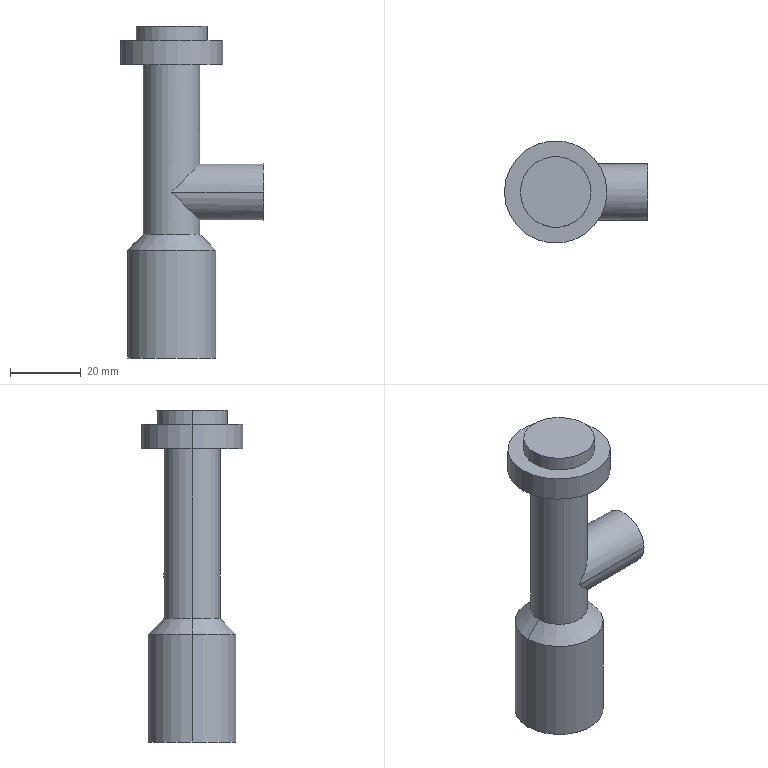Part | STEP file | ASND-0110-Body 1-15 | 1 solid | 17 faces | box 40.5 x 29 x 94 mm | volume 35874 mm3 | cylinder 10 | plane 5 | cone 2 | commonest cylinder face diameters 16 x4 20 x2 25 x2 29 x2
STEP:
#1=CARTESIAN_POINT('',(0.,0.,0.));
#2=DIRECTION('',(0.,0.,1.));
#3=DIRECTION('',(1.,0.,0.));
#4=AXIS2_PLACEMENT_3D('',#1,#2,#3);
#5=CARTESIAN_POINT('',(8.,0.,35.));
#6=VERTEX_POINT('',#5);
#7=CARTESIAN_POINT('',(-8.,0.,35.));
#8=VERTEX_POINT('',#7);
#9=CARTESIAN_POINT('',(0.,0.,35.));
#10=DIRECTION('',(0.,0.,-1.));
#11=DIRECTION('',(-1.,0.,0.));
#12=AXIS2_PLACEMENT_3D('',#9,#10,#11);
#13=CIRCLE('',#12,8.);
#14=CARTESIAN_POINT('',(0.,0.,35.));
#15=DIRECTION('',(0.,0.,1.));
#16=DIRECTION('',(-1.,0.,0.));
#17=AXIS2_PLACEMENT_3D('',#14,#15,#16);
#18=CYLINDRICAL_SURFACE('',#17,8.);
#19=CARTESIAN_POINT('',(6.283,0.));
#20=DIRECTION('',(-1.,0.));
#21=VECTOR('',#20,1.);
#22=LINE('',#19,#21);
#23=(GEOMETRIC_REPRESENTATION_CONTEXT(2)PARAMETRIC_REPRESENTATION_CONTEXT()REPRESENTATION_CONTEXT('',''));
#24=DEFINITIONAL_REPRESENTATION('',(#22),#23);
#25=PCURVE('',#18,#24);
#26=CARTESIAN_POINT('',(0.,0.,32.75));
#27=DIRECTION('',(0.,0.,-1.));
#28=DIRECTION('',(-1.,0.,0.));
#29=AXIS2_PLACEMENT_3D('',#26,#27,#28);
#30=CONICAL_SURFACE('',#29,10.25,0.7854);
#31=CARTESIAN_POINT('',(0.,-2.25));
#32=DIRECTION('',(1.,0.));
#33=VECTOR('',#32,1.);
#34=LINE('',#31,#33);
#35=(GEOMETRIC_REPRESENTATION_CONTEXT(2)PARAMETRIC_REPRESENTATION_CONTEXT()REPRESENTATION_CONTEXT('',''));
#36=DEFINITIONAL_REPRESENTATION('',(#34),#35);
#37=PCURVE('',#30,#36);
#38=SURFACE_CURVE('',#13,(#25,#37),.PCURVE_S1.);
#39=EDGE_CURVE('',#6,#8,#38,.T.);
#40=ORIENTED_EDGE('',*,*,#39,.F.);
#41=CARTESIAN_POINT('',(8.,0.,39.));
#42=VERTEX_POINT('',#41);
#43=CARTESIAN_POINT('',(8.,0.,35.));
#44=DIRECTION('',(0.,0.,1.));
#45=VECTOR('',#44,1.);
#46=LINE('',#43,#45);
#47=CARTESIAN_POINT('',(3.142,0.));
#48=DIRECTION('',(0.,1.));
#49=VECTOR('',#48,1.);
#50=LINE('',#47,#49);
#51=(GEOMETRIC_REPRESENTATION_CONTEXT(2)PARAMETRIC_REPRESENTATION_CONTEXT()REPRESENTATION_CONTEXT('',''));
#52=DEFINITIONAL_REPRESENTATION('',(#50),#51);
#53=PCURVE('',#18,#52);
#54=CARTESIAN_POINT('',(0.,0.,35.));
#55=DIRECTION('',(0.,0.,1.));
#56=DIRECTION('',(-1.,0.,0.));
#57=AXIS2_PLACEMENT_3D('',#54,#55,#56);
#58=CYLINDRICAL_SURFACE('',#57,8.);
#59=CARTESIAN_POINT('',(3.142,0.));
#60=DIRECTION('',(0.,1.));
#61=VECTOR('',#60,1.);
#62=LINE('',#59,#61);
#63=(GEOMETRIC_REPRESENTATION_CONTEXT(2)PARAMETRIC_REPRESENTATION_CONTEXT()REPRESENTATION_CONTEXT('',''));
#64=DEFINITIONAL_REPRESENTATION('',(#62),#63);
#65=PCURVE('',#58,#64);
#66=SURFACE_CURVE('',#46,(#53,#65),.PCURVE_S1.);
#67=EDGE_CURVE('',#6,#42,#66,.T.);
#68=ORIENTED_EDGE('',*,*,#67,.T.);
#69=CARTESIAN_POINT('',(0.,-8.,47.));
#70=VERTEX_POINT('',#69);
#71=CARTESIAN_POINT('',(8.,0.,39.));
#72=CARTESIAN_POINT('',(8.,-4.686,39.));
#73=CARTESIAN_POINT('',(4.686,-8.,42.314));
#74=CARTESIAN_POINT('',(0.,-8.,47.));
#75=(BOUNDED_CURVE()B_SPLINE_CURVE(3,(#71,#72,#73,#74),.UNSPECIFIED.,.F.,.F.)B_SPLINE_CURVE_WITH_KNOTS((4,4),(0.,1.571),.PIECEWISE_BEZIER_KNOTS.)CURVE()GEOMETRIC_REPRESENTATION_ITEM()RATIONAL_B_SPLINE_CURVE((1.,0.8047,0.8047,1.))REPRESENTATION_ITEM(''));
#76=CARTESIAN_POINT('',(3.142,4.));
#77=CARTESIAN_POINT('',(3.12,4.));
#78=CARTESIAN_POINT('',(3.077,4.011));
#79=CARTESIAN_POINT('',(3.01,4.063));
#80=CARTESIAN_POINT('',(2.942,4.153));
#81=CARTESIAN_POINT('',(2.872,4.283));
#82=CARTESIAN_POINT('',(2.801,4.454));
#83=CARTESIAN_POINT('',(2.729,4.666));
#84=CARTESIAN_POINT('',(2.655,4.921));
#85=CARTESIAN_POINT('',(2.581,5.217));
#86=CARTESIAN_POINT('',(2.507,5.553));
#87=CARTESIAN_POINT('',(2.432,5.928));
#88=CARTESIAN_POINT('',(2.356,6.338));
#89=CARTESIAN_POINT('',(2.281,6.78));
#90=CARTESIAN_POINT('',(2.206,7.25));
#91=CARTESIAN_POINT('',(2.131,7.744));
#92=CARTESIAN_POINT('',(2.057,8.258));
#93=CARTESIAN_POINT('',(1.984,8.786));
#94=CARTESIAN_POINT('',(1.912,9.324));
#95=CARTESIAN_POINT('',(1.841,9.867));
#96=CARTESIAN_POINT('',(1.771,10.41));
#97=CARTESIAN_POINT('',(1.702,10.949));
#98=CARTESIAN_POINT('',(1.636,11.481));
#99=CARTESIAN_POINT('',(1.592,11.829));
#100=CARTESIAN_POINT('',(1.571,12.));
#101=B_SPLINE_CURVE_WITH_KNOTS('',3,(#76,#77,#78,#79,#80,#81,#82,#83,#84,#85,#86,#87,#88,#89,#90,#91,#92,#93,#94,#95,#96,#97,#98,#99,#100),.UNSPECIFIED.,.F.,.F.,(4,1,1,1,1,1,1,1,1,1,1,1,1,1,1,1,1,1,1,1,1,1,4),(0.,0.0714,0.1428,0.2142,0.2856,0.357,0.4284,0.4998,0.5712,0.6426,0.714,0.7854,0.8568,0.9282,0.9996,1.071,1.142,1.214,1.285,1.357,1.428,1.499,1.571),.UNSPECIFIED.);
#102=(GEOMETRIC_REPRESENTATION_CONTEXT(2)PARAMETRIC_REPRESENTATION_CONTEXT()REPRESENTATION_CONTEXT('',''));
#103=DEFINITIONAL_REPRESENTATION('',(#101),#102);
#104=PCURVE('',#18,#103);
#105=CARTESIAN_POINT('',(0.,0.,47.));
#106=DIRECTION('',(1.,0.,0.));
#107=DIRECTION('',(0.,-1.,0.));
#108=AXIS2_PLACEMENT_3D('',#105,#106,#107);
#109=CYLINDRICAL_SURFACE('',#108,8.);
#110=CARTESIAN_POINT('',(1.571,8.));
#111=CARTESIAN_POINT('',(1.549,8.));
#112=CARTESIAN_POINT('',(1.506,7.989));
#113=CARTESIAN_POINT('',(1.439,7.937));
#114=CARTESIAN_POINT('',(1.371,7.847));
#115=CARTESIAN_POINT('',(1.301,7.717));
#116=CARTESIAN_POINT('',(1.23,7.546));
#117=CARTESIAN_POINT('',(1.158,7.334));
#118=CARTESIAN_POINT('',(1.085,7.079));
#119=CARTESIAN_POINT('',(1.01,6.783));
#120=CARTESIAN_POINT('',(0.9358,6.447));
#121=CARTESIAN_POINT('',(0.8607,6.072));
#122=CARTESIAN_POINT('',(0.7854,5.662));
#123=CARTESIAN_POINT('',(0.7101,5.22));
#124=CARTESIAN_POINT('',(0.635,4.75));
#125=CARTESIAN_POINT('',(0.5603,4.256));
#126=CARTESIAN_POINT('',(0.4863,3.742));
#127=CARTESIAN_POINT('',(0.413,3.214));
#128=CARTESIAN_POINT('',(0.3408,2.676));
#129=CARTESIAN_POINT('',(0.2697,2.133));
#130=CARTESIAN_POINT('',(0.2,1.59));
#131=CARTESIAN_POINT('',(0.1316,1.051));
#132=CARTESIAN_POINT('',(0.06485,0.5189));
#133=CARTESIAN_POINT('',(0.02143,0.1714));
#134=CARTESIAN_POINT('',(0.,0.));
#135=B_SPLINE_CURVE_WITH_KNOTS('',3,(#110,#111,#112,#113,#114,#115,#116,#117,#118,#119,#120,#121,#122,#123,#124,#125,#126,#127,#128,#129,#130,#131,#132,#133,#134),.UNSPECIFIED.,.F.,.F.,(4,1,1,1,1,1,1,1,1,1,1,1,1,1,1,1,1,1,1,1,1,1,4),(0.,0.0714,0.1428,0.2142,0.2856,0.357,0.4284,0.4998,0.5712,0.6426,0.714,0.7854,0.8568,0.9282,0.9996,1.071,1.142,1.214,1.285,1.357,1.428,1.499,1.571),.UNSPECIFIED.);
#136=(GEOMETRIC_REPRESENTATION_CONTEXT(2)PARAMETRIC_REPRESENTATION_CONTEXT()REPRESENTATION_CONTEXT('',''));
#137=DEFINITIONAL_REPRESENTATION('',(#135),#136);
#138=PCURVE('',#109,#137);
#139=SURFACE_CURVE('',#75,(#104,#138),.PCURVE_S1.);
#140=EDGE_CURVE('',#42,#70,#139,.T.);
#141=ORIENTED_EDGE('',*,*,#140,.T.);
#142=CARTESIAN_POINT('',(8.,0.,55.));
#143=VERTEX_POINT('',#142);
#144=CARTESIAN_POINT('',(0.,-8.,47.));
#145=CARTESIAN_POINT('',(4.686,-8.,51.686));
#146=CARTESIAN_POINT('',(8.,-4.686,55.));
#147=CARTESIAN_POINT('',(8.,0.,55.));
#148=(BOUNDED_CURVE()B_SPLINE_CURVE(3,(#144,#145,#146,#147),.UNSPECIFIED.,.F.,.F.)B_SPLINE_CURVE_WITH_KNOTS((4,4),(1.571,3.142),.PIECEWISE_BEZIER_KNOTS.)CURVE()GEOMETRIC_REPRESENTATION_ITEM()RATIONAL_B_SPLINE_CURVE((1.,0.8047,0.8047,1.))REPRESENTATION_ITEM(''));
#149=CARTESIAN_POINT('',(1.571,12.));
#150=CARTESIAN_POINT('',(1.592,12.171));
#151=CARTESIAN_POINT('',(1.636,12.519));
#152=CARTESIAN_POINT('',(1.702,13.051));
#153=CARTESIAN_POINT('',(1.771,13.59));
#154=CARTESIAN_POINT('',(1.841,14.133));
#155=CARTESIAN_POINT('',(1.912,14.676));
#156=CARTESIAN_POINT('',(1.984,15.214));
#157=CARTESIAN_POINT('',(2.057,15.742));
#158=CARTESIAN_POINT('',(2.131,16.256));
#159=CARTESIAN_POINT('',(2.206,16.75));
#160=CARTESIAN_POINT('',(2.281,17.22));
#161=CARTESIAN_POINT('',(2.356,17.662));
#162=CARTESIAN_POINT('',(2.432,18.072));
#163=CARTESIAN_POINT('',(2.507,18.447));
#164=CARTESIAN_POINT('',(2.581,18.783));
#165=CARTESIAN_POINT('',(2.655,19.079));
#166=CARTESIAN_POINT('',(2.729,19.334));
#167=CARTESIAN_POINT('',(2.801,19.546));
#168=CARTESIAN_POINT('',(2.872,19.717));
#169=CARTESIAN_POINT('',(2.942,19.847));
#170=CARTESIAN_POINT('',(3.01,19.937));
#171=CARTESIAN_POINT('',(3.077,19.989));
#172=CARTESIAN_POINT('',(3.12,20.));
#173=CARTESIAN_POINT('',(3.142,20.));
#174=B_SPLINE_CURVE_WITH_KNOTS('',3,(#149,#150,#151,#152,#153,#154,#155,#156,#157,#158,#159,#160,#161,#162,#163,#164,#165,#166,#167,#168,#169,#170,#171,#172,#173),.UNSPECIFIED.,.F.,.F.,(4,1,1,1,1,1,1,1,1,1,1,1,1,1,1,1,1,1,1,1,1,1,4),(1.571,1.642,1.714,1.785,1.856,1.928,1.999,2.071,2.142,2.213,2.285,2.356,2.428,2.499,2.57,2.642,2.713,2.785,2.856,2.927,2.999,3.07,3.142),.QUASI_UNIFORM_KNOTS.);
#175=(GEOMETRIC_REPRESENTATION_CONTEXT(2)PARAMETRIC_REPRESENTATION_CONTEXT()REPRESENTATION_CONTEXT('',''));
#176=DEFINITIONAL_REPRESENTATION('',(#174),#175);
#177=PCURVE('',#18,#176);
#178=CARTESIAN_POINT('',(0.,0.,47.));
#179=DIRECTION('',(1.,0.,0.));
#180=DIRECTION('',(0.,-1.,0.));
#181=AXIS2_PLACEMENT_3D('',#178,#179,#180);
#182=CYLINDRICAL_SURFACE('',#181,8.);
#183=CARTESIAN_POINT('',(6.283,0.));
#184=CARTESIAN_POINT('',(6.262,0.1714));
#185=CARTESIAN_POINT('',(6.218,0.5189));
#186=CARTESIAN_POINT('',(6.152,1.051));
#187=CARTESIAN_POINT('',(6.083,1.59));
#188=CARTESIAN_POINT('',(6.013,2.133));
#189=CARTESIAN_POINT('',(5.942,2.676));
#190=CARTESIAN_POINT('',(5.87,3.214));
#191=CARTESIAN_POINT('',(5.797,3.742));
#192=CARTESIAN_POINT('',(5.723,4.256));
#193=CARTESIAN_POINT('',(5.648,4.75));
#194=CARTESIAN_POINT('',(5.573,5.22));
#195=CARTESIAN_POINT('',(5.498,5.662));
#196=CARTESIAN_POINT('',(5.422,6.072));
#197=CARTESIAN_POINT('',(5.347,6.447));
#198=CARTESIAN_POINT('',(5.273,6.783));
#199=CARTESIAN_POINT('',(5.199,7.079));
#200=CARTESIAN_POINT('',(5.125,7.334));
#201=CARTESIAN_POINT('',(5.053,7.546));
#202=CARTESIAN_POINT('',(4.982,7.717));
#203=CARTESIAN_POINT('',(4.912,7.847));
#204=CARTESIAN_POINT('',(4.844,7.937));
#205=CARTESIAN_POINT('',(4.777,7.989));
#206=CARTESIAN_POINT('',(4.734,8.));
#207=CARTESIAN_POINT('',(4.712,8.));
#208=B_SPLINE_CURVE_WITH_KNOTS('',3,(#183,#184,#185,#186,#187,#188,#189,#190,#191,#192,#193,#194,#195,#196,#197,#198,#199,#200,#201,#202,#203,#204,#205,#206,#207),.UNSPECIFIED.,.F.,.F.,(4,1,1,1,1,1,1,1,1,1,1,1,1,1,1,1,1,1,1,1,1,1,4),(1.571,1.642,1.714,1.785,1.856,1.928,1.999,2.071,2.142,2.213,2.285,2.356,2.428,2.499,2.57,2.642,2.713,2.785,2.856,2.927,2.999,3.07,3.142),.QUASI_UNIFORM_KNOTS.);
#209=(GEOMETRIC_REPRESENTATION_CONTEXT(2)PARAMETRIC_REPRESENTATION_CONTEXT()REPRESENTATION_CONTEXT('',''));
#210=DEFINITIONAL_REPRESENTATION('',(#208),#209);
#211=PCURVE('',#182,#210);
#212=SURFACE_CURVE('',#148,(#177,#211),.PCURVE_S1.);
#213=EDGE_CURVE('',#70,#143,#212,.T.);
#214=ORIENTED_EDGE('',*,*,#213,.T.);
#215=CARTESIAN_POINT('',(8.,0.,83.));
#216=VERTEX_POINT('',#215);
#217=CARTESIAN_POINT('',(8.,0.,35.));
#218=DIRECTION('',(0.,0.,1.));
#219=VECTOR('',#218,1.);
#220=LINE('',#217,#219);
#221=CARTESIAN_POINT('',(3.142,0.));
#222=DIRECTION('',(0.,1.));
#223=VECTOR('',#222,1.);
#224=LINE('',#221,#223);
#225=(GEOMETRIC_REPRESENTATION_CONTEXT(2)PARAMETRIC_REPRESENTATION_CONTEXT()REPRESENTATION_CONTEXT('',''));
#226=DEFINITIONAL_REPRESENTATION('',(#224),#225);
#227=PCURVE('',#18,#226);
#228=CARTESIAN_POINT('',(3.142,0.));
#229=DIRECTION('',(0.,1.));
#230=VECTOR('',#229,1.);
#231=LINE('',#228,#230);
#232=(GEOMETRIC_REPRESENTATION_CONTEXT(2)PARAMETRIC_REPRESENTATION_CONTEXT()REPRESENTATION_CONTEXT('',''));
#233=DEFINITIONAL_REPRESENTATION('',(#231),#232);
#234=PCURVE('',#58,#233);
#235=SURFACE_CURVE('',#220,(#227,#234),.PCURVE_S1.);
#236=EDGE_CURVE('',#143,#216,#235,.T.);
#237=ORIENTED_EDGE('',*,*,#236,.T.);
#238=CARTESIAN_POINT('',(-8.,0.,83.));
#239=VERTEX_POINT('',#238);
#240=CARTESIAN_POINT('',(0.,0.,83.));
#241=DIRECTION('',(0.,0.,-1.));
#242=DIRECTION('',(-1.,0.,0.));
#243=AXIS2_PLACEMENT_3D('',#240,#241,#242);
#244=CIRCLE('',#243,8.);
#245=CARTESIAN_POINT('',(6.283,48.));
#246=DIRECTION('',(-1.,0.));
#247=VECTOR('',#246,1.);
#248=LINE('',#245,#247);
#249=(GEOMETRIC_REPRESENTATION_CONTEXT(2)PARAMETRIC_REPRESENTATION_CONTEXT()REPRESENTATION_CONTEXT('',''));
#250=DEFINITIONAL_REPRESENTATION('',(#248),#249);
#251=PCURVE('',#18,#250);
#252=CARTESIAN_POINT('',(0.,0.,83.));
#253=DIRECTION('',(0.,0.,-1.));
#254=DIRECTION('',(0.7071,0.7071,0.));
#255=AXIS2_PLACEMENT_3D('',#252,#253,#254);
#256=PLANE('',#255);
#257=CARTESIAN_POINT('',(0.,0.));
#258=DIRECTION('',(-0.7071,-0.7071));
#259=AXIS2_PLACEMENT_2D('',#257,#258);
#260=CIRCLE('',#259,8.);
#261=(GEOMETRIC_REPRESENTATION_CONTEXT(2)PARAMETRIC_REPRESENTATION_CONTEXT()REPRESENTATION_CONTEXT('',''));
#262=DEFINITIONAL_REPRESENTATION('',(#260),#261);
#263=PCURVE('',#256,#262);
#264=SURFACE_CURVE('',#244,(#251,#263),.PCURVE_S1.);
#265=EDGE_CURVE('',#216,#239,#264,.T.);
#266=ORIENTED_EDGE('',*,*,#265,.T.);
#267=CARTESIAN_POINT('',(-8.,0.,35.));
#268=DIRECTION('',(0.,0.,1.));
#269=VECTOR('',#268,1.);
#270=LINE('',#267,#269);
#271=CARTESIAN_POINT('',(0.,0.));
#272=DIRECTION('',(0.,1.));
#273=VECTOR('',#272,1.);
#274=LINE('',#271,#273);
#275=(GEOMETRIC_REPRESENTATION_CONTEXT(2)PARAMETRIC_REPRESENTATION_CONTEXT()REPRESENTATION_CONTEXT('',''));
#276=DEFINITIONAL_REPRESENTATION('',(#274),#275);
#277=PCURVE('',#18,#276);
#278=CARTESIAN_POINT('',(6.283,0.));
#279=DIRECTION('',(0.,1.));
#280=VECTOR('',#279,1.);
#281=LINE('',#278,#280);
#282=(GEOMETRIC_REPRESENTATION_CONTEXT(2)PARAMETRIC_REPRESENTATION_CONTEXT()REPRESENTATION_CONTEXT('',''));
#283=DEFINITIONAL_REPRESENTATION('',(#281),#282);
#284=PCURVE('',#58,#283);
#285=SURFACE_CURVE('',#270,(#277,#284),.PCURVE_S1.);
#286=EDGE_CURVE('',#8,#239,#285,.T.);
#287=ORIENTED_EDGE('',*,*,#286,.F.);
#288=EDGE_LOOP('',(#40,#68,#141,#214,#237,#266,#287));
#289=FACE_BOUND('',#288,.T.);
#290=ADVANCED_FACE('',(#289),#18,.T.);
#291=CARTESIAN_POINT('',(12.5,0.,0.));
#292=VERTEX_POINT('',#291);
#293=CARTESIAN_POINT('',(-12.5,0.,0.));
#294=VERTEX_POINT('',#293);
#295=CARTESIAN_POINT('',(0.,0.,0.));
#296=DIRECTION('',(0.,0.,-1.));
#297=DIRECTION('',(-1.,0.,0.));
#298=AXIS2_PLACEMENT_3D('',#295,#296,#297);
#299=CIRCLE('',#298,12.5);
#300=CARTESIAN_POINT('',(0.,0.,0.));
#301=DIRECTION('',(0.,0.,1.));
#302=DIRECTION('',(-1.,0.,0.));
#303=AXIS2_PLACEMENT_3D('',#300,#301,#302);
#304=CYLINDRICAL_SURFACE('',#303,12.5);
#305=CARTESIAN_POINT('',(6.283,0.));
#306=DIRECTION('',(-1.,0.));
#307=VECTOR('',#306,1.);
#308=LINE('',#305,#307);
#309=(GEOMETRIC_REPRESENTATION_CONTEXT(2)PARAMETRIC_REPRESENTATION_CONTEXT()REPRESENTATION_CONTEXT('',''));
#310=DEFINITIONAL_REPRESENTATION('',(#308),#309);
#311=PCURVE('',#304,#310);
#312=CARTESIAN_POINT('',(0.,0.,0.));
#313=DIRECTION('',(0.,0.,-1.));
#314=DIRECTION('',(0.7071,0.7071,0.));
#315=AXIS2_PLACEMENT_3D('',#312,#313,#314);
#316=PLANE('',#315);
#317=CARTESIAN_POINT('',(0.,0.));
#318=DIRECTION('',(-0.7071,-0.7071));
#319=AXIS2_PLACEMENT_2D('',#317,#318);
#320=CIRCLE('',#319,12.5);
#321=(GEOMETRIC_REPRESENTATION_CONTEXT(2)PARAMETRIC_REPRESENTATION_CONTEXT()REPRESENTATION_CONTEXT('',''));
#322=DEFINITIONAL_REPRESENTATION('',(#320),#321);
#323=PCURVE('',#316,#322);
#324=SURFACE_CURVE('',#299,(#311,#323),.PCURVE_S1.);
#325=EDGE_CURVE('',#292,#294,#324,.T.);
#326=ORIENTED_EDGE('',*,*,#325,.F.);
#327=CARTESIAN_POINT('',(12.5,0.,30.5));
#328=VERTEX_POINT('',#327);
#329=CARTESIAN_POINT('',(12.5,0.,0.));
#330=DIRECTION('',(0.,0.,1.));
#331=VECTOR('',#330,1.);
#332=LINE('',#329,#331);
#333=CARTESIAN_POINT('',(3.142,0.));
#334=DIRECTION('',(0.,1.));
#335=VECTOR('',#334,1.);
#336=LINE('',#333,#335);
#337=(GEOMETRIC_REPRESENTATION_CONTEXT(2)PARAMETRIC_REPRESENTATION_CONTEXT()REPRESENTATION_CONTEXT('',''));
#338=DEFINITIONAL_REPRESENTATION('',(#336),#337);
#339=PCURVE('',#304,#338);
#340=CARTESIAN_POINT('',(0.,0.,0.));
#341=DIRECTION('',(0.,0.,1.));
#342=DIRECTION('',(-1.,0.,0.));
#343=AXIS2_PLACEMENT_3D('',#340,#341,#342);
#344=CYLINDRICAL_SURFACE('',#343,12.5);
#345=CARTESIAN_POINT('',(3.142,0.));
#346=DIRECTION('',(0.,1.));
#347=VECTOR('',#346,1.);
#348=LINE('',#345,#347);
#349=(GEOMETRIC_REPRESENTATION_CONTEXT(2)PARAMETRIC_REPRESENTATION_CONTEXT()REPRESENTATION_CONTEXT('',''));
#350=DEFINITIONAL_REPRESENTATION('',(#348),#349);
#351=PCURVE('',#344,#350);
#352=SURFACE_CURVE('',#332,(#339,#351),.PCURVE_S1.);
#353=EDGE_CURVE('',#292,#328,#352,.T.);
#354=ORIENTED_EDGE('',*,*,#353,.T.);
#355=CARTESIAN_POINT('',(-12.5,0.,30.5));
#356=VERTEX_POINT('',#355);
#357=CARTESIAN_POINT('',(0.,0.,30.5));
#358=DIRECTION('',(0.,0.,1.));
#359=DIRECTION('',(-1.,0.,0.));
#360=AXIS2_PLACEMENT_3D('',#357,#358,#359);
#361=CIRCLE('',#360,12.5);
#362=CARTESIAN_POINT('',(0.,30.5));
#363=DIRECTION('',(1.,0.));
#364=VECTOR('',#363,1.);
#365=LINE('',#362,#364);
#366=(GEOMETRIC_REPRESENTATION_CONTEXT(2)PARAMETRIC_REPRESENTATION_CONTEXT()REPRESENTATION_CONTEXT('',''));
#367=DEFINITIONAL_REPRESENTATION('',(#365),#366);
#368=PCURVE('',#304,#367);
#369=CARTESIAN_POINT('',(6.283,2.25));
#370=DIRECTION('',(-1.,0.));
#371=VECTOR('',#370,1.);
#372=LINE('',#369,#371);
#373=(GEOMETRIC_REPRESENTATION_CONTEXT(2)PARAMETRIC_REPRESENTATION_CONTEXT()REPRESENTATION_CONTEXT('',''));
#374=DEFINITIONAL_REPRESENTATION('',(#372),#373);
#375=PCURVE('',#30,#374);
#376=SURFACE_CURVE('',#361,(#368,#375),.PCURVE_S1.);
#377=EDGE_CURVE('',#356,#328,#376,.T.);
#378=ORIENTED_EDGE('',*,*,#377,.F.);
#379=CARTESIAN_POINT('',(-12.5,0.,0.));
#380=DIRECTION('',(0.,0.,1.));
#381=VECTOR('',#380,1.);
#382=LINE('',#379,#381);
#383=CARTESIAN_POINT('',(0.,0.));
#384=DIRECTION('',(0.,1.));
#385=VECTOR('',#384,1.);
#386=LINE('',#383,#385);
#387=(GEOMETRIC_REPRESENTATION_CONTEXT(2)PARAMETRIC_REPRESENTATION_CONTEXT()REPRESENTATION_CONTEXT('',''));
#388=DEFINITIONAL_REPRESENTATION('',(#386),#387);
#389=PCURVE('',#304,#388);
#390=CARTESIAN_POINT('',(6.283,0.));
#391=DIRECTION('',(0.,1.));
#392=VECTOR('',#391,1.);
#393=LINE('',#390,#392);
#394=(GEOMETRIC_REPRESENTATION_CONTEXT(2)PARAMETRIC_REPRESENTATION_CONTEXT()REPRESENTATION_CONTEXT('',''));
#395=DEFINITIONAL_REPRESENTATION('',(#393),#394);
#396=PCURVE('',#344,#395);
#397=SURFACE_CURVE('',#382,(#389,#396),.PCURVE_S1.);
#398=EDGE_CURVE('',#294,#356,#397,.T.);
#399=ORIENTED_EDGE('',*,*,#398,.F.);
#400=EDGE_LOOP('',(#326,#354,#378,#399));
#401=FACE_BOUND('',#400,.T.);
#402=ADVANCED_FACE('',(#401),#304,.T.);
#403=CARTESIAN_POINT('',(0.,0.,35.));
#404=DIRECTION('',(0.,0.,-1.));
#405=DIRECTION('',(-1.,0.,0.));
#406=AXIS2_PLACEMENT_3D('',#403,#404,#405);
#407=CIRCLE('',#406,8.);
#408=CARTESIAN_POINT('',(0.,0.,32.75));
#409=DIRECTION('',(0.,0.,-1.));
#410=DIRECTION('',(-1.,0.,0.));
#411=AXIS2_PLACEMENT_3D('',#408,#409,#410);
#412=CONICAL_SURFACE('',#411,10.25,0.7854);
#413=CARTESIAN_POINT('',(0.,-2.25));
#414=DIRECTION('',(1.,0.));
#415=VECTOR('',#414,1.);
#416=LINE('',#413,#415);
#417=(GEOMETRIC_REPRESENTATION_CONTEXT(2)PARAMETRIC_REPRESENTATION_CONTEXT()REPRESENTATION_CONTEXT('',''));
#418=DEFINITIONAL_REPRESENTATION('',(#416),#417);
#419=PCURVE('',#412,#418);
#420=CARTESIAN_POINT('',(6.283,0.));
#421=DIRECTION('',(-1.,0.));
#422=VECTOR('',#421,1.);
#423=LINE('',#420,#422);
#424=(GEOMETRIC_REPRESENTATION_CONTEXT(2)PARAMETRIC_REPRESENTATION_CONTEXT()REPRESENTATION_CONTEXT('',''));
#425=DEFINITIONAL_REPRESENTATION('',(#423),#424);
#426=PCURVE('',#58,#425);
#427=SURFACE_CURVE('',#407,(#419,#426),.PCURVE_S1.);
#428=EDGE_CURVE('',#8,#6,#427,.T.);
#429=ORIENTED_EDGE('',*,*,#428,.T.);
#430=CARTESIAN_POINT('',(10.25,0.,32.75));
#431=DIRECTION('',(0.7071,0.,-0.7071));
#432=VECTOR('',#431,1.);
#433=LINE('',#430,#432);
#434=CARTESIAN_POINT('',(3.142,0.));
#435=DIRECTION('',(0.,1.));
#436=VECTOR('',#435,1.);
#437=LINE('',#434,#436);
#438=(GEOMETRIC_REPRESENTATION_CONTEXT(2)PARAMETRIC_REPRESENTATION_CONTEXT()REPRESENTATION_CONTEXT('',''));
#439=DEFINITIONAL_REPRESENTATION('',(#437),#438);
#440=PCURVE('',#412,#439);
#441=CARTESIAN_POINT('',(3.142,0.));
#442=DIRECTION('',(0.,1.));
#443=VECTOR('',#442,1.);
#444=LINE('',#441,#443);
#445=(GEOMETRIC_REPRESENTATION_CONTEXT(2)PARAMETRIC_REPRESENTATION_CONTEXT()REPRESENTATION_CONTEXT('',''));
#446=DEFINITIONAL_REPRESENTATION('',(#444),#445);
#447=PCURVE('',#30,#446);
#448=SURFACE_CURVE('',#433,(#440,#447),.PCURVE_S1.);
#449=EDGE_CURVE('',#6,#328,#448,.T.);
#450=ORIENTED_EDGE('',*,*,#449,.T.);
#451=CARTESIAN_POINT('',(0.,0.,30.5));
#452=DIRECTION('',(0.,0.,1.));
#453=DIRECTION('',(-1.,0.,0.));
#454=AXIS2_PLACEMENT_3D('',#451,#452,#453);
#455=CIRCLE('',#454,12.5);
#456=CARTESIAN_POINT('',(6.283,2.25));
#457=DIRECTION('',(-1.,0.));
#458=VECTOR('',#457,1.);
#459=LINE('',#456,#458);
#460=(GEOMETRIC_REPRESENTATION_CONTEXT(2)PARAMETRIC_REPRESENTATION_CONTEXT()REPRESENTATION_CONTEXT('',''));
#461=DEFINITIONAL_REPRESENTATION('',(#459),#460);
#462=PCURVE('',#412,#461);
#463=CARTESIAN_POINT('',(0.,30.5));
#464=DIRECTION('',(1.,0.));
#465=VECTOR('',#464,1.);
#466=LINE('',#463,#465);
#467=(GEOMETRIC_REPRESENTATION_CONTEXT(2)PARAMETRIC_REPRESENTATION_CONTEXT()REPRESENTATION_CONTEXT('',''));
#468=DEFINITIONAL_REPRESENTATION('',(#466),#467);
#469=PCURVE('',#344,#468);
#470=SURFACE_CURVE('',#455,(#462,#469),.PCURVE_S1.);
#471=EDGE_CURVE('',#328,#356,#470,.T.);
#472=ORIENTED_EDGE('',*,*,#471,.T.);
#473=CARTESIAN_POINT('',(-10.25,0.,32.75));
#474=DIRECTION('',(-0.7071,0.,-0.7071));
#475=VECTOR('',#474,1.);
#476=LINE('',#473,#475);
#477=CARTESIAN_POINT('',(0.,0.));
#478=DIRECTION('',(0.,1.));
#479=VECTOR('',#478,1.);
#480=LINE('',#477,#479);
#481=(GEOMETRIC_REPRESENTATION_CONTEXT(2)PARAMETRIC_REPRESENTATION_CONTEXT()REPRESENTATION_CONTEXT('',''));
#482=DEFINITIONAL_REPRESENTATION('',(#480),#481);
#483=PCURVE('',#412,#482);
#484=CARTESIAN_POINT('',(6.283,0.));
#485=DIRECTION('',(0.,1.));
#486=VECTOR('',#485,1.);
#487=LINE('',#484,#486);
#488=(GEOMETRIC_REPRESENTATION_CONTEXT(2)PARAMETRIC_REPRESENTATION_CONTEXT()REPRESENTATION_CONTEXT('',''));
#489=DEFINITIONAL_REPRESENTATION('',(#487),#488);
#490=PCURVE('',#30,#489);
#491=SURFACE_CURVE('',#476,(#483,#490),.PCURVE_S1.);
#492=EDGE_CURVE('',#8,#356,#491,.T.);
#493=ORIENTED_EDGE('',*,*,#492,.F.);
#494=EDGE_LOOP('',(#429,#450,#472,#493));
#495=FACE_BOUND('',#494,.T.);
#496=ADVANCED_FACE('',(#495),#412,.T.);
#497=CARTESIAN_POINT('',(-14.5,0.,90.));
#498=VERTEX_POINT('',#497);
#499=CARTESIAN_POINT('',(14.5,0.,90.));
#500=VERTEX_POINT('',#499);
#501=CARTESIAN_POINT('',(0.,0.,90.));
#502=DIRECTION('',(0.,0.,-1.));
#503=DIRECTION('',(-1.,0.,0.));
#504=AXIS2_PLACEMENT_3D('',#501,#502,#503);
#505=CIRCLE('',#504,14.5);
#506=CARTESIAN_POINT('',(0.,0.,90.));
#507=DIRECTION('',(0.,0.,-1.));
#508=DIRECTION('',(-1.,0.,0.));
#509=AXIS2_PLACEMENT_3D('',#506,#507,#508);
#510=CYLINDRICAL_SURFACE('',#509,14.5);
#511=CARTESIAN_POINT('',(0.,0.));
#512=DIRECTION('',(1.,0.));
#513=VECTOR('',#512,1.);
#514=LINE('',#511,#513);
#515=(GEOMETRIC_REPRESENTATION_CONTEXT(2)PARAMETRIC_REPRESENTATION_CONTEXT()REPRESENTATION_CONTEXT('',''));
#516=DEFINITIONAL_REPRESENTATION('',(#514),#515);
#517=PCURVE('',#510,#516);
#518=CARTESIAN_POINT('',(0.,0.,90.));
#519=DIRECTION('',(0.,0.,-1.));
#520=DIRECTION('',(0.7071,0.7071,0.));
#521=AXIS2_PLACEMENT_3D('',#518,#519,#520);
#522=PLANE('',#521);
#523=CARTESIAN_POINT('',(0.,0.));
#524=DIRECTION('',(-0.7071,-0.7071));
#525=AXIS2_PLACEMENT_2D('',#523,#524);
#526=CIRCLE('',#525,14.5);
#527=(GEOMETRIC_REPRESENTATION_CONTEXT(2)PARAMETRIC_REPRESENTATION_CONTEXT()REPRESENTATION_CONTEXT('',''));
#528=DEFINITIONAL_REPRESENTATION('',(#526),#527);
#529=PCURVE('',#522,#528);
#530=SURFACE_CURVE('',#505,(#517,#529),.PCURVE_S1.);
#531=EDGE_CURVE('',#498,#500,#530,.T.);
#532=ORIENTED_EDGE('',*,*,#531,.T.);
#533=CARTESIAN_POINT('',(14.5,0.,83.));
#534=VERTEX_POINT('',#533);
#535=CARTESIAN_POINT('',(14.5,0.,90.));
#536=DIRECTION('',(0.,0.,-1.));
#537=VECTOR('',#536,1.);
#538=LINE('',#535,#537);
#539=CARTESIAN_POINT('',(3.142,0.));
#540=DIRECTION('',(0.,1.));
#541=VECTOR('',#540,1.);
#542=LINE('',#539,#541);
#543=(GEOMETRIC_REPRESENTATION_CONTEXT(2)PARAMETRIC_REPRESENTATION_CONTEXT()REPRESENTATION_CONTEXT('',''));
#544=DEFINITIONAL_REPRESENTATION('',(#542),#543);
#545=PCURVE('',#510,#544);
#546=CARTESIAN_POINT('',(0.,0.,90.));
#547=DIRECTION('',(0.,0.,-1.));
#548=DIRECTION('',(-1.,0.,0.));
#549=AXIS2_PLACEMENT_3D('',#546,#547,#548);
#550=CYLINDRICAL_SURFACE('',#549,14.5);
#551=CARTESIAN_POINT('',(3.142,0.));
#552=DIRECTION('',(0.,1.));
#553=VECTOR('',#552,1.);
#554=LINE('',#551,#553);
#555=(GEOMETRIC_REPRESENTATION_CONTEXT(2)PARAMETRIC_REPRESENTATION_CONTEXT()REPRESENTATION_CONTEXT('',''));
#556=DEFINITIONAL_REPRESENTATION('',(#554),#555);
#557=PCURVE('',#550,#556);
#558=SURFACE_CURVE('',#538,(#545,#557),.PCURVE_S1.);
#559=EDGE_CURVE('',#500,#534,#558,.T.);
#560=ORIENTED_EDGE('',*,*,#559,.T.);
#561=CARTESIAN_POINT('',(-14.5,0.,83.));
#562=VERTEX_POINT('',#561);
#563=CARTESIAN_POINT('',(0.,0.,83.));
#564=DIRECTION('',(0.,0.,1.));
#565=DIRECTION('',(-1.,0.,0.));
#566=AXIS2_PLACEMENT_3D('',#563,#564,#565);
#567=CIRCLE('',#566,14.5);
#568=CARTESIAN_POINT('',(6.283,7.));
#569=DIRECTION('',(-1.,0.));
#570=VECTOR('',#569,1.);
#571=LINE('',#568,#570);
#572=(GEOMETRIC_REPRESENTATION_CONTEXT(2)PARAMETRIC_REPRESENTATION_CONTEXT()REPRESENTATION_CONTEXT('',''));
#573=DEFINITIONAL_REPRESENTATION('',(#571),#572);
#574=PCURVE('',#510,#573);
#575=CARTESIAN_POINT('',(-10.253,-10.253));
#576=CARTESIAN_POINT('',(-28.012,7.506));
#577=CARTESIAN_POINT('',(-3.753,14.006));
#578=CARTESIAN_POINT('',(20.506,20.506));
#579=CARTESIAN_POINT('',(14.006,-3.753));
#580=CARTESIAN_POINT('',(7.506,-28.012));
#581=CARTESIAN_POINT('',(-10.253,-10.253));
#582=(BOUNDED_CURVE()B_SPLINE_CURVE(2,(#575,#576,#577,#578,#579,#580,#581),.UNSPECIFIED.,.T.,.F.)B_SPLINE_CURVE_WITH_KNOTS((1,2,2,2,2,1),(-2.094,0.,2.094,4.189,6.283,8.378),.UNSPECIFIED.)CURVE()GEOMETRIC_REPRESENTATION_ITEM()RATIONAL_B_SPLINE_CURVE((1.,0.5,1.,0.5,1.,0.5,1.))REPRESENTATION_ITEM(''));
#583=(GEOMETRIC_REPRESENTATION_CONTEXT(2)PARAMETRIC_REPRESENTATION_CONTEXT()REPRESENTATION_CONTEXT('',''));
#584=DEFINITIONAL_REPRESENTATION('',(#582),#583);
#585=PCURVE('',#256,#584);
#586=SURFACE_CURVE('',#567,(#574,#585),.PCURVE_S1.);
#587=EDGE_CURVE('',#534,#562,#586,.T.);
#588=ORIENTED_EDGE('',*,*,#587,.T.);
#589=CARTESIAN_POINT('',(-14.5,0.,90.));
#590=DIRECTION('',(0.,0.,-1.));
#591=VECTOR('',#590,1.);
#592=LINE('',#589,#591);
#593=CARTESIAN_POINT('',(0.,0.));
#594=DIRECTION('',(0.,1.));
#595=VECTOR('',#594,1.);
#596=LINE('',#593,#595);
#597=(GEOMETRIC_REPRESENTATION_CONTEXT(2)PARAMETRIC_REPRESENTATION_CONTEXT()REPRESENTATION_CONTEXT('',''));
#598=DEFINITIONAL_REPRESENTATION('',(#596),#597);
#599=PCURVE('',#510,#598);
#600=CARTESIAN_POINT('',(6.283,0.));
#601=DIRECTION('',(0.,1.));
#602=VECTOR('',#601,1.);
#603=LINE('',#600,#602);
#604=(GEOMETRIC_REPRESENTATION_CONTEXT(2)PARAMETRIC_REPRESENTATION_CONTEXT()REPRESENTATION_CONTEXT('',''));
#605=DEFINITIONAL_REPRESENTATION('',(#603),#604);
#606=PCURVE('',#550,#605);
#607=SURFACE_CURVE('',#592,(#599,#606),.PCURVE_S1.);
#608=EDGE_CURVE('',#498,#562,#607,.T.);
#609=ORIENTED_EDGE('',*,*,#608,.F.);
#610=EDGE_LOOP('',(#532,#560,#588,#609));
#611=FACE_BOUND('',#610,.T.);
#612=ADVANCED_FACE('',(#611),#510,.T.);
#613=CARTESIAN_POINT('',(10.,0.,90.));
#614=VERTEX_POINT('',#613);
#615=CARTESIAN_POINT('',(-10.,0.,90.));
#616=VERTEX_POINT('',#615);
#617=CARTESIAN_POINT('',(0.,0.,90.));
#618=DIRECTION('',(0.,0.,-1.));
#619=DIRECTION('',(-1.,0.,0.));
#620=AXIS2_PLACEMENT_3D('',#617,#618,#619);
#621=CIRCLE('',#620,10.);
#622=CARTESIAN_POINT('',(0.,0.,90.));
#623=DIRECTION('',(0.,0.,1.));
#624=DIRECTION('',(-1.,0.,0.));
#625=AXIS2_PLACEMENT_3D('',#622,#623,#624);
#626=CYLINDRICAL_SURFACE('',#625,10.);
#627=CARTESIAN_POINT('',(6.283,0.));
#628=DIRECTION('',(-1.,0.));
#629=VECTOR('',#628,1.);
#630=LINE('',#627,#629);
#631=(GEOMETRIC_REPRESENTATION_CONTEXT(2)PARAMETRIC_REPRESENTATION_CONTEXT()REPRESENTATION_CONTEXT('',''));
#632=DEFINITIONAL_REPRESENTATION('',(#630),#631);
#633=PCURVE('',#626,#632);
#634=CARTESIAN_POINT('',(0.,0.));
#635=DIRECTION('',(-0.7071,-0.7071));
#636=AXIS2_PLACEMENT_2D('',#634,#635);
#637=CIRCLE('',#636,10.);
#638=(GEOMETRIC_REPRESENTATION_CONTEXT(2)PARAMETRIC_REPRESENTATION_CONTEXT()REPRESENTATION_CONTEXT('',''));
#639=DEFINITIONAL_REPRESENTATION('',(#637),#638);
#640=PCURVE('',#522,#639);
#641=SURFACE_CURVE('',#621,(#633,#640),.PCURVE_S1.);
#642=EDGE_CURVE('',#614,#616,#641,.T.);
#643=ORIENTED_EDGE('',*,*,#642,.F.);
#644=CARTESIAN_POINT('',(10.,0.,94.));
#645=VERTEX_POINT('',#644);
#646=CARTESIAN_POINT('',(10.,0.,90.));
#647=DIRECTION('',(0.,0.,1.));
#648=VECTOR('',#647,1.);
#649=LINE('',#646,#648);
#650=CARTESIAN_POINT('',(3.142,0.));
#651=DIRECTION('',(0.,1.));
#652=VECTOR('',#651,1.);
#653=LINE('',#650,#652);
#654=(GEOMETRIC_REPRESENTATION_CONTEXT(2)PARAMETRIC_REPRESENTATION_CONTEXT()REPRESENTATION_CONTEXT('',''));
#655=DEFINITIONAL_REPRESENTATION('',(#653),#654);
#656=PCURVE('',#626,#655);
#657=CARTESIAN_POINT('',(0.,0.,90.));
#658=DIRECTION('',(0.,0.,1.));
#659=DIRECTION('',(-1.,0.,0.));
#660=AXIS2_PLACEMENT_3D('',#657,#658,#659);
#661=CYLINDRICAL_SURFACE('',#660,10.);
#662=CARTESIAN_POINT('',(3.142,0.));
#663=DIRECTION('',(0.,1.));
#664=VECTOR('',#663,1.);
#665=LINE('',#662,#664);
#666=(GEOMETRIC_REPRESENTATION_CONTEXT(2)PARAMETRIC_REPRESENTATION_CONTEXT()REPRESENTATION_CONTEXT('',''));
#667=DEFINITIONAL_REPRESENTATION('',(#665),#666);
#668=PCURVE('',#661,#667);
#669=SURFACE_CURVE('',#649,(#656,#668),.PCURVE_S1.);
#670=EDGE_CURVE('',#614,#645,#669,.T.);
#671=ORIENTED_EDGE('',*,*,#670,.T.);
#672=CARTESIAN_POINT('',(-10.,0.,94.));
#673=VERTEX_POINT('',#672);
#674=CARTESIAN_POINT('',(0.,0.,94.));
#675=DIRECTION('',(0.,0.,-1.));
#676=DIRECTION('',(-1.,0.,0.));
#677=AXIS2_PLACEMENT_3D('',#674,#675,#676);
#678=CIRCLE('',#677,10.);
#679=CARTESIAN_POINT('',(6.283,4.));
#680=DIRECTION('',(-1.,0.));
#681=VECTOR('',#680,1.);
#682=LINE('',#679,#681);
#683=(GEOMETRIC_REPRESENTATION_CONTEXT(2)PARAMETRIC_REPRESENTATION_CONTEXT()REPRESENTATION_CONTEXT('',''));
#684=DEFINITIONAL_REPRESENTATION('',(#682),#683);
#685=PCURVE('',#626,#684);
#686=CARTESIAN_POINT('',(0.,0.,94.));
#687=DIRECTION('',(0.,0.,-1.));
#688=DIRECTION('',(0.7071,0.7071,0.));
#689=AXIS2_PLACEMENT_3D('',#686,#687,#688);
#690=PLANE('',#689);
#691=CARTESIAN_POINT('',(0.,0.));
#692=DIRECTION('',(-0.7071,-0.7071));
#693=AXIS2_PLACEMENT_2D('',#691,#692);
#694=CIRCLE('',#693,10.);
#695=(GEOMETRIC_REPRESENTATION_CONTEXT(2)PARAMETRIC_REPRESENTATION_CONTEXT()REPRESENTATION_CONTEXT('',''));
#696=DEFINITIONAL_REPRESENTATION('',(#694),#695);
#697=PCURVE('',#690,#696);
#698=SURFACE_CURVE('',#678,(#685,#697),.PCURVE_S1.);
#699=EDGE_CURVE('',#645,#673,#698,.T.);
#700=ORIENTED_EDGE('',*,*,#699,.T.);
#701=CARTESIAN_POINT('',(-10.,0.,90.));
#702=DIRECTION('',(0.,0.,1.));
#703=VECTOR('',#702,1.);
#704=LINE('',#701,#703);
#705=CARTESIAN_POINT('',(0.,0.));
#706=DIRECTION('',(0.,1.));
#707=VECTOR('',#706,1.);
#708=LINE('',#705,#707);
#709=(GEOMETRIC_REPRESENTATION_CONTEXT(2)PARAMETRIC_REPRESENTATION_CONTEXT()REPRESENTATION_CONTEXT('',''));
#710=DEFINITIONAL_REPRESENTATION('',(#708),#709);
#711=PCURVE('',#626,#710);
#712=CARTESIAN_POINT('',(6.283,0.));
#713=DIRECTION('',(0.,1.));
#714=VECTOR('',#713,1.);
#715=LINE('',#712,#714);
#716=(GEOMETRIC_REPRESENTATION_CONTEXT(2)PARAMETRIC_REPRESENTATION_CONTEXT()REPRESENTATION_CONTEXT('',''));
#717=DEFINITIONAL_REPRESENTATION('',(#715),#716);
#718=PCURVE('',#661,#717);
#719=SURFACE_CURVE('',#704,(#711,#718),.PCURVE_S1.);
#720=EDGE_CURVE('',#616,#673,#719,.T.);
#721=ORIENTED_EDGE('',*,*,#720,.F.);
#722=EDGE_LOOP('',(#643,#671,#700,#721));
#723=FACE_BOUND('',#722,.T.);
#724=ADVANCED_FACE('',(#723),#626,.T.);
#725=CARTESIAN_POINT('',(0.,8.,47.));
#726=VERTEX_POINT('',#725);
#727=CARTESIAN_POINT('',(0.,8.,47.));
#728=CARTESIAN_POINT('',(4.686,8.,42.314));
#729=CARTESIAN_POINT('',(8.,4.686,39.));
#730=CARTESIAN_POINT('',(8.,0.,39.));
#731=(BOUNDED_CURVE()B_SPLINE_CURVE(3,(#727,#728,#729,#730),.UNSPECIFIED.,.F.,.F.)B_SPLINE_CURVE_WITH_KNOTS((4,4),(4.712,6.283),.PIECEWISE_BEZIER_KNOTS.)CURVE()GEOMETRIC_REPRESENTATION_ITEM()RATIONAL_B_SPLINE_CURVE((1.,0.8047,0.8047,1.))REPRESENTATION_ITEM(''));
#732=CARTESIAN_POINT('',(3.142,0.));
#733=CARTESIAN_POINT('',(3.12,0.1714));
#734=CARTESIAN_POINT('',(3.077,0.5189));
#735=CARTESIAN_POINT('',(3.01,1.051));
#736=CARTESIAN_POINT('',(2.942,1.59));
#737=CARTESIAN_POINT('',(2.872,2.133));
#738=CARTESIAN_POINT('',(2.801,2.676));
#739=CARTESIAN_POINT('',(2.729,3.214));
#740=CARTESIAN_POINT('',(2.655,3.742));
#741=CARTESIAN_POINT('',(2.581,4.256));
#742=CARTESIAN_POINT('',(2.507,4.75));
#743=CARTESIAN_POINT('',(2.432,5.22));
#744=CARTESIAN_POINT('',(2.356,5.662));
#745=CARTESIAN_POINT('',(2.281,6.072));
#746=CARTESIAN_POINT('',(2.206,6.447));
#747=CARTESIAN_POINT('',(2.131,6.783));
#748=CARTESIAN_POINT('',(2.057,7.079));
#749=CARTESIAN_POINT('',(1.984,7.334));
#750=CARTESIAN_POINT('',(1.912,7.546));
#751=CARTESIAN_POINT('',(1.841,7.717));
#752=CARTESIAN_POINT('',(1.771,7.847));
#753=CARTESIAN_POINT('',(1.702,7.937));
#754=CARTESIAN_POINT('',(1.636,7.989));
#755=CARTESIAN_POINT('',(1.592,8.));
#756=CARTESIAN_POINT('',(1.571,8.));
#757=B_SPLINE_CURVE_WITH_KNOTS('',3,(#732,#733,#734,#735,#736,#737,#738,#739,#740,#741,#742,#743,#744,#745,#746,#747,#748,#749,#750,#751,#752,#753,#754,#755,#756),.UNSPECIFIED.,.F.,.F.,(4,1,1,1,1,1,1,1,1,1,1,1,1,1,1,1,1,1,1,1,1,1,4),(4.712,4.784,4.855,4.927,4.998,5.069,5.141,5.212,5.284,5.355,5.426,5.498,5.569,5.641,5.712,5.783,5.855,5.926,5.998,6.069,6.14,6.212,6.283),.QUASI_UNIFORM_KNOTS.);
#758=(GEOMETRIC_REPRESENTATION_CONTEXT(2)PARAMETRIC_REPRESENTATION_CONTEXT()REPRESENTATION_CONTEXT('',''));
#759=DEFINITIONAL_REPRESENTATION('',(#757),#758);
#760=PCURVE('',#109,#759);
#761=CARTESIAN_POINT('',(4.712,12.));
#762=CARTESIAN_POINT('',(4.691,11.829));
#763=CARTESIAN_POINT('',(4.648,11.481));
#764=CARTESIAN_POINT('',(4.581,10.949));
#765=CARTESIAN_POINT('',(4.512,10.41));
#766=CARTESIAN_POINT('',(4.443,9.867));
#767=CARTESIAN_POINT('',(4.372,9.324));
#768=CARTESIAN_POINT('',(4.299,8.786));
#769=CARTESIAN_POINT('',(4.226,8.258));
#770=CARTESIAN_POINT('',(4.152,7.744));
#771=CARTESIAN_POINT('',(4.077,7.25));
#772=CARTESIAN_POINT('',(4.002,6.78));
#773=CARTESIAN_POINT('',(3.927,6.338));
#774=CARTESIAN_POINT('',(3.852,5.928));
#775=CARTESIAN_POINT('',(3.777,5.553));
#776=CARTESIAN_POINT('',(3.702,5.217));
#777=CARTESIAN_POINT('',(3.628,4.921));
#778=CARTESIAN_POINT('',(3.555,4.666));
#779=CARTESIAN_POINT('',(3.482,4.454));
#780=CARTESIAN_POINT('',(3.411,4.283));
#781=CARTESIAN_POINT('',(3.342,4.153));
#782=CARTESIAN_POINT('',(3.273,4.063));
#783=CARTESIAN_POINT('',(3.206,4.011));
#784=CARTESIAN_POINT('',(3.163,4.));
#785=CARTESIAN_POINT('',(3.142,4.));
#786=B_SPLINE_CURVE_WITH_KNOTS('',3,(#761,#762,#763,#764,#765,#766,#767,#768,#769,#770,#771,#772,#773,#774,#775,#776,#777,#778,#779,#780,#781,#782,#783,#784,#785),.UNSPECIFIED.,.F.,.F.,(4,1,1,1,1,1,1,1,1,1,1,1,1,1,1,1,1,1,1,1,1,1,4),(4.712,4.784,4.855,4.927,4.998,5.069,5.141,5.212,5.284,5.355,5.426,5.498,5.569,5.641,5.712,5.783,5.855,5.926,5.998,6.069,6.14,6.212,6.283),.QUASI_UNIFORM_KNOTS.);
#787=(GEOMETRIC_REPRESENTATION_CONTEXT(2)PARAMETRIC_REPRESENTATION_CONTEXT()REPRESENTATION_CONTEXT('',''));
#788=DEFINITIONAL_REPRESENTATION('',(#786),#787);
#789=PCURVE('',#58,#788);
#790=SURFACE_CURVE('',#731,(#760,#789),.PCURVE_S1.);
#791=EDGE_CURVE('',#726,#42,#790,.T.);
#792=ORIENTED_EDGE('',*,*,#791,.F.);
#793=CARTESIAN_POINT('',(26.,8.,47.));
#794=VERTEX_POINT('',#793);
#795=CARTESIAN_POINT('',(0.,8.,47.));
#796=DIRECTION('',(1.,0.,0.));
#797=VECTOR('',#796,1.);
#798=LINE('',#795,#797);
#799=CARTESIAN_POINT('',(3.142,0.));
#800=DIRECTION('',(0.,1.));
#801=VECTOR('',#800,1.);
#802=LINE('',#799,#801);
#803=(GEOMETRIC_REPRESENTATION_CONTEXT(2)PARAMETRIC_REPRESENTATION_CONTEXT()REPRESENTATION_CONTEXT('',''));
#804=DEFINITIONAL_REPRESENTATION('',(#802),#803);
#805=PCURVE('',#109,#804);
#806=CARTESIAN_POINT('',(3.142,0.));
#807=DIRECTION('',(0.,1.));
#808=VECTOR('',#807,1.);
#809=LINE('',#806,#808);
#810=(GEOMETRIC_REPRESENTATION_CONTEXT(2)PARAMETRIC_REPRESENTATION_CONTEXT()REPRESENTATION_CONTEXT('',''));
#811=DEFINITIONAL_REPRESENTATION('',(#809),#810);
#812=PCURVE('',#182,#811);
#813=SURFACE_CURVE('',#798,(#805,#812),.PCURVE_S1.);
#814=EDGE_CURVE('',#726,#794,#813,.T.);
#815=ORIENTED_EDGE('',*,*,#814,.T.);
#816=CARTESIAN_POINT('',(26.,-8.,47.));
#817=VERTEX_POINT('',#816);
#818=CARTESIAN_POINT('',(26.,0.,47.));
#819=DIRECTION('',(-1.,0.,0.));
#820=DIRECTION('',(0.,-1.,0.));
#821=AXIS2_PLACEMENT_3D('',#818,#819,#820);
#822=CIRCLE('',#821,8.);
#823=CARTESIAN_POINT('',(6.283,26.));
#824=DIRECTION('',(-1.,0.));
#825=VECTOR('',#824,1.);
#826=LINE('',#823,#825);
#827=(GEOMETRIC_REPRESENTATION_CONTEXT(2)PARAMETRIC_REPRESENTATION_CONTEXT()REPRESENTATION_CONTEXT('',''));
#828=DEFINITIONAL_REPRESENTATION('',(#826),#827);
#829=PCURVE('',#109,#828);
#830=CARTESIAN_POINT('',(26.,0.,47.));
#831=DIRECTION('',(-1.,0.,0.));
#832=DIRECTION('',(0.,0.7071,0.7071));
#833=AXIS2_PLACEMENT_3D('',#830,#831,#832);
#834=PLANE('',#833);
#835=CARTESIAN_POINT('',(0.,0.));
#836=DIRECTION('',(-0.7071,-0.7071));
#837=AXIS2_PLACEMENT_2D('',#835,#836);
#838=CIRCLE('',#837,8.);
#839=(GEOMETRIC_REPRESENTATION_CONTEXT(2)PARAMETRIC_REPRESENTATION_CONTEXT()REPRESENTATION_CONTEXT('',''));
#840=DEFINITIONAL_REPRESENTATION('',(#838),#839);
#841=PCURVE('',#834,#840);
#842=SURFACE_CURVE('',#822,(#829,#841),.PCURVE_S1.);
#843=EDGE_CURVE('',#794,#817,#842,.T.);
#844=ORIENTED_EDGE('',*,*,#843,.T.);
#845=CARTESIAN_POINT('',(0.,-8.,47.));
#846=DIRECTION('',(1.,0.,0.));
#847=VECTOR('',#846,1.);
#848=LINE('',#845,#847);
#849=CARTESIAN_POINT('',(0.,0.));
#850=DIRECTION('',(0.,1.));
#851=VECTOR('',#850,1.);
#852=LINE('',#849,#851);
#853=(GEOMETRIC_REPRESENTATION_CONTEXT(2)PARAMETRIC_REPRESENTATION_CONTEXT()REPRESENTATION_CONTEXT('',''));
#854=DEFINITIONAL_REPRESENTATION('',(#852),#853);
#855=PCURVE('',#109,#854);
#856=CARTESIAN_POINT('',(6.283,0.));
#857=DIRECTION('',(0.,1.));
#858=VECTOR('',#857,1.);
#859=LINE('',#856,#858);
#860=(GEOMETRIC_REPRESENTATION_CONTEXT(2)PARAMETRIC_REPRESENTATION_CONTEXT()REPRESENTATION_CONTEXT('',''));
#861=DEFINITIONAL_REPRESENTATION('',(#859),#860);
#862=PCURVE('',#182,#861);
#863=SURFACE_CURVE('',#848,(#855,#862),.PCURVE_S1.);
#864=EDGE_CURVE('',#70,#817,#863,.T.);
#865=ORIENTED_EDGE('',*,*,#864,.F.);
#866=ORIENTED_EDGE('',*,*,#140,.F.);
#867=EDGE_LOOP('',(#792,#815,#844,#865,#866));
#868=FACE_BOUND('',#867,.T.);
#869=ADVANCED_FACE('',(#868),#109,.T.);
#870=ORIENTED_EDGE('',*,*,#814,.F.);
#871=CARTESIAN_POINT('',(8.,0.,55.));
#872=CARTESIAN_POINT('',(8.,4.686,55.));
#873=CARTESIAN_POINT('',(4.686,8.,51.686));
#874=CARTESIAN_POINT('',(0.,8.,47.));
#875=(BOUNDED_CURVE()B_SPLINE_CURVE(3,(#871,#872,#873,#874),.UNSPECIFIED.,.F.,.F.)B_SPLINE_CURVE_WITH_KNOTS((4,4),(3.142,4.712),.PIECEWISE_BEZIER_KNOTS.)CURVE()GEOMETRIC_REPRESENTATION_ITEM()RATIONAL_B_SPLINE_CURVE((1.,0.8047,0.8047,1.))REPRESENTATION_ITEM(''));
#876=CARTESIAN_POINT('',(4.712,8.));
#877=CARTESIAN_POINT('',(4.691,8.));
#878=CARTESIAN_POINT('',(4.648,7.989));
#879=CARTESIAN_POINT('',(4.581,7.937));
#880=CARTESIAN_POINT('',(4.512,7.847));
#881=CARTESIAN_POINT('',(4.443,7.717));
#882=CARTESIAN_POINT('',(4.372,7.546));
#883=CARTESIAN_POINT('',(4.299,7.334));
#884=CARTESIAN_POINT('',(4.226,7.079));
#885=CARTESIAN_POINT('',(4.152,6.783));
#886=CARTESIAN_POINT('',(4.077,6.447));
#887=CARTESIAN_POINT('',(4.002,6.072));
#888=CARTESIAN_POINT('',(3.927,5.662));
#889=CARTESIAN_POINT('',(3.852,5.22));
#890=CARTESIAN_POINT('',(3.777,4.75));
#891=CARTESIAN_POINT('',(3.702,4.256));
#892=CARTESIAN_POINT('',(3.628,3.742));
#893=CARTESIAN_POINT('',(3.555,3.214));
#894=CARTESIAN_POINT('',(3.482,2.676));
#895=CARTESIAN_POINT('',(3.411,2.133));
#896=CARTESIAN_POINT('',(3.342,1.59));
#897=CARTESIAN_POINT('',(3.273,1.051));
#898=CARTESIAN_POINT('',(3.206,0.5189));
#899=CARTESIAN_POINT('',(3.163,0.1714));
#900=CARTESIAN_POINT('',(3.142,0.));
#901=B_SPLINE_CURVE_WITH_KNOTS('',3,(#876,#877,#878,#879,#880,#881,#882,#883,#884,#885,#886,#887,#888,#889,#890,#891,#892,#893,#894,#895,#896,#897,#898,#899,#900),.UNSPECIFIED.,.F.,.F.,(4,1,1,1,1,1,1,1,1,1,1,1,1,1,1,1,1,1,1,1,1,1,4),(3.142,3.213,3.284,3.356,3.427,3.499,3.57,3.641,3.713,3.784,3.856,3.927,3.998,4.07,4.141,4.213,4.284,4.355,4.427,4.498,4.57,4.641,4.712),.QUASI_UNIFORM_KNOTS.);
#902=(GEOMETRIC_REPRESENTATION_CONTEXT(2)PARAMETRIC_REPRESENTATION_CONTEXT()REPRESENTATION_CONTEXT('',''));
#903=DEFINITIONAL_REPRESENTATION('',(#901),#902);
#904=PCURVE('',#182,#903);
#905=CARTESIAN_POINT('',(3.142,20.));
#906=CARTESIAN_POINT('',(3.163,20.));
#907=CARTESIAN_POINT('',(3.206,19.989));
#908=CARTESIAN_POINT('',(3.273,19.937));
#909=CARTESIAN_POINT('',(3.342,19.847));
#910=CARTESIAN_POINT('',(3.411,19.717));
#911=CARTESIAN_POINT('',(3.482,19.546));
#912=CARTESIAN_POINT('',(3.555,19.334));
#913=CARTESIAN_POINT('',(3.628,19.079));
#914=CARTESIAN_POINT('',(3.702,18.783));
#915=CARTESIAN_POINT('',(3.777,18.447));
#916=CARTESIAN_POINT('',(3.852,18.072));
#917=CARTESIAN_POINT('',(3.927,17.662));
#918=CARTESIAN_POINT('',(4.002,17.22));
#919=CARTESIAN_POINT('',(4.077,16.75));
#920=CARTESIAN_POINT('',(4.152,16.256));
#921=CARTESIAN_POINT('',(4.226,15.742));
#922=CARTESIAN_POINT('',(4.299,15.214));
#923=CARTESIAN_POINT('',(4.372,14.676));
#924=CARTESIAN_POINT('',(4.443,14.133));
#925=CARTESIAN_POINT('',(4.512,13.59));
#926=CARTESIAN_POINT('',(4.581,13.051));
#927=CARTESIAN_POINT('',(4.648,12.519));
#928=CARTESIAN_POINT('',(4.691,12.171));
#929=CARTESIAN_POINT('',(4.712,12.));
#930=B_SPLINE_CURVE_WITH_KNOTS('',3,(#905,#906,#907,#908,#909,#910,#911,#912,#913,#914,#915,#916,#917,#918,#919,#920,#921,#922,#923,#924,#925,#926,#927,#928,#929),.UNSPECIFIED.,.F.,.F.,(4,1,1,1,1,1,1,1,1,1,1,1,1,1,1,1,1,1,1,1,1,1,4),(3.142,3.213,3.284,3.356,3.427,3.499,3.57,3.641,3.713,3.784,3.856,3.927,3.998,4.07,4.141,4.213,4.284,4.355,4.427,4.498,4.57,4.641,4.712),.QUASI_UNIFORM_KNOTS.);
#931=(GEOMETRIC_REPRESENTATION_CONTEXT(2)PARAMETRIC_REPRESENTATION_CONTEXT()REPRESENTATION_CONTEXT('',''));
#932=DEFINITIONAL_REPRESENTATION('',(#930),#931);
#933=PCURVE('',#58,#932);
#934=SURFACE_CURVE('',#875,(#904,#933),.PCURVE_S1.);
#935=EDGE_CURVE('',#143,#726,#934,.T.);
#936=ORIENTED_EDGE('',*,*,#935,.F.);
#937=ORIENTED_EDGE('',*,*,#213,.F.);
#938=ORIENTED_EDGE('',*,*,#864,.T.);
#939=CARTESIAN_POINT('',(26.,0.,47.));
#940=DIRECTION('',(-1.,0.,0.));
#941=DIRECTION('',(0.,-1.,0.));
#942=AXIS2_PLACEMENT_3D('',#939,#940,#941);
#943=CIRCLE('',#942,8.);
#944=CARTESIAN_POINT('',(6.283,26.));
#945=DIRECTION('',(-1.,0.));
#946=VECTOR('',#945,1.);
#947=LINE('',#944,#946);
#948=(GEOMETRIC_REPRESENTATION_CONTEXT(2)PARAMETRIC_REPRESENTATION_CONTEXT()REPRESENTATION_CONTEXT('',''));
#949=DEFINITIONAL_REPRESENTATION('',(#947),#948);
#950=PCURVE('',#182,#949);
#951=CARTESIAN_POINT('',(0.,0.));
#952=DIRECTION('',(-0.7071,-0.7071));
#953=AXIS2_PLACEMENT_2D('',#951,#952);
#954=CIRCLE('',#953,8.);
#955=(GEOMETRIC_REPRESENTATION_CONTEXT(2)PARAMETRIC_REPRESENTATION_CONTEXT()REPRESENTATION_CONTEXT('',''));
#956=DEFINITIONAL_REPRESENTATION('',(#954),#955);
#957=PCURVE('',#834,#956);
#958=SURFACE_CURVE('',#943,(#950,#957),.PCURVE_S1.);
#959=EDGE_CURVE('',#817,#794,#958,.T.);
#960=ORIENTED_EDGE('',*,*,#959,.T.);
#961=EDGE_LOOP('',(#870,#936,#937,#938,#960));
#962=FACE_BOUND('',#961,.T.);
#963=ADVANCED_FACE('',(#962),#182,.T.);
#964=ORIENTED_EDGE('',*,*,#959,.F.);
#965=ORIENTED_EDGE('',*,*,#843,.F.);
#966=EDGE_LOOP('',(#964,#965));
#967=FACE_BOUND('',#966,.T.);
#968=ADVANCED_FACE('',(#967),#834,.F.);
#969=ORIENTED_EDGE('',*,*,#670,.F.);
#970=CARTESIAN_POINT('',(0.,0.,90.));
#971=DIRECTION('',(0.,0.,-1.));
#972=DIRECTION('',(-1.,0.,0.));
#973=AXIS2_PLACEMENT_3D('',#970,#971,#972);
#974=CIRCLE('',#973,10.);
#975=CARTESIAN_POINT('',(6.283,0.));
#976=DIRECTION('',(-1.,0.));
#977=VECTOR('',#976,1.);
#978=LINE('',#975,#977);
#979=(GEOMETRIC_REPRESENTATION_CONTEXT(2)PARAMETRIC_REPRESENTATION_CONTEXT()REPRESENTATION_CONTEXT('',''));
#980=DEFINITIONAL_REPRESENTATION('',(#978),#979);
#981=PCURVE('',#661,#980);
#982=CARTESIAN_POINT('',(0.,0.));
#983=DIRECTION('',(-0.7071,-0.7071));
#984=AXIS2_PLACEMENT_2D('',#982,#983);
#985=CIRCLE('',#984,10.);
#986=(GEOMETRIC_REPRESENTATION_CONTEXT(2)PARAMETRIC_REPRESENTATION_CONTEXT()REPRESENTATION_CONTEXT('',''));
#987=DEFINITIONAL_REPRESENTATION('',(#985),#986);
#988=PCURVE('',#522,#987);
#989=SURFACE_CURVE('',#974,(#981,#988),.PCURVE_S1.);
#990=EDGE_CURVE('',#616,#614,#989,.T.);
#991=ORIENTED_EDGE('',*,*,#990,.F.);
#992=ORIENTED_EDGE('',*,*,#720,.T.);
#993=CARTESIAN_POINT('',(0.,0.,94.));
#994=DIRECTION('',(0.,0.,-1.));
#995=DIRECTION('',(-1.,0.,0.));
#996=AXIS2_PLACEMENT_3D('',#993,#994,#995);
#997=CIRCLE('',#996,10.);
#998=CARTESIAN_POINT('',(6.283,4.));
#999=DIRECTION('',(-1.,0.));
#1000=VECTOR('',#999,1.);
#1001=LINE('',#998,#1000);
#1002=(GEOMETRIC_REPRESENTATION_CONTEXT(2)PARAMETRIC_REPRESENTATION_CONTEXT()REPRESENTATION_CONTEXT('',''));
#1003=DEFINITIONAL_REPRESENTATION('',(#1001),#1002);
#1004=PCURVE('',#661,#1003);
#1005=CARTESIAN_POINT('',(0.,0.));
#1006=DIRECTION('',(-0.7071,-0.7071));
#1007=AXIS2_PLACEMENT_2D('',#1005,#1006);
#1008=CIRCLE('',#1007,10.);
#1009=(GEOMETRIC_REPRESENTATION_CONTEXT(2)PARAMETRIC_REPRESENTATION_CONTEXT()REPRESENTATION_CONTEXT('',''));
#1010=DEFINITIONAL_REPRESENTATION('',(#1008),#1009);
#1011=PCURVE('',#690,#1010);
#1012=SURFACE_CURVE('',#997,(#1004,#1011),.PCURVE_S1.);
#1013=EDGE_CURVE('',#673,#645,#1012,.T.);
#1014=ORIENTED_EDGE('',*,*,#1013,.T.);
#1015=EDGE_LOOP('',(#969,#991,#992,#1014));
#1016=FACE_BOUND('',#1015,.T.);
#1017=ADVANCED_FACE('',(#1016),#661,.T.);
#1018=ORIENTED_EDGE('',*,*,#1013,.F.);
#1019=ORIENTED_EDGE('',*,*,#699,.F.);
#1020=EDGE_LOOP('',(#1018,#1019));
#1021=FACE_BOUND('',#1020,.T.);
#1022=ADVANCED_FACE('',(#1021),#690,.F.);
#1023=ORIENTED_EDGE('',*,*,#559,.F.);
#1024=CARTESIAN_POINT('',(0.,0.,90.));
#1025=DIRECTION('',(0.,0.,-1.));
#1026=DIRECTION('',(-1.,0.,0.));
#1027=AXIS2_PLACEMENT_3D('',#1024,#1025,#1026);
#1028=CIRCLE('',#1027,14.5);
#1029=CARTESIAN_POINT('',(0.,0.));
#1030=DIRECTION('',(1.,0.));
#1031=VECTOR('',#1030,1.);
#1032=LINE('',#1029,#1031);
#1033=(GEOMETRIC_REPRESENTATION_CONTEXT(2)PARAMETRIC_REPRESENTATION_CONTEXT()REPRESENTATION_CONTEXT('',''));
#1034=DEFINITIONAL_REPRESENTATION('',(#1032),#1033);
#1035=PCURVE('',#550,#1034);
#1036=CARTESIAN_POINT('',(0.,0.));
#1037=DIRECTION('',(-0.7071,-0.7071));
#1038=AXIS2_PLACEMENT_2D('',#1036,#1037);
#1039=CIRCLE('',#1038,14.5);
#1040=(GEOMETRIC_REPRESENTATION_CONTEXT(2)PARAMETRIC_REPRESENTATION_CONTEXT()REPRESENTATION_CONTEXT('',''));
#1041=DEFINITIONAL_REPRESENTATION('',(#1039),#1040);
#1042=PCURVE('',#522,#1041);
#1043=SURFACE_CURVE('',#1028,(#1035,#1042),.PCURVE_S1.);
#1044=EDGE_CURVE('',#500,#498,#1043,.T.);
#1045=ORIENTED_EDGE('',*,*,#1044,.T.);
#1046=ORIENTED_EDGE('',*,*,#608,.T.);
#1047=CARTESIAN_POINT('',(0.,0.,83.));
#1048=DIRECTION('',(0.,0.,1.));
#1049=DIRECTION('',(-1.,0.,0.));
#1050=AXIS2_PLACEMENT_3D('',#1047,#1048,#1049);
#1051=CIRCLE('',#1050,14.5);
#1052=CARTESIAN_POINT('',(6.283,7.));
#1053=DIRECTION('',(-1.,0.));
#1054=VECTOR('',#1053,1.);
#1055=LINE('',#1052,#1054);
#1056=(GEOMETRIC_REPRESENTATION_CONTEXT(2)PARAMETRIC_REPRESENTATION_CONTEXT()REPRESENTATION_CONTEXT('',''));
#1057=DEFINITIONAL_REPRESENTATION('',(#1055),#1056);
#1058=PCURVE('',#550,#1057);
#1059=CARTESIAN_POINT('',(-10.253,-10.253));
#1060=CARTESIAN_POINT('',(-28.012,7.506));
#1061=CARTESIAN_POINT('',(-3.753,14.006));
#1062=CARTESIAN_POINT('',(20.506,20.506));
#1063=CARTESIAN_POINT('',(14.006,-3.753));
#1064=CARTESIAN_POINT('',(7.506,-28.012));
#1065=CARTESIAN_POINT('',(-10.253,-10.253));
#1066=(BOUNDED_CURVE()B_SPLINE_CURVE(2,(#1059,#1060,#1061,#1062,#1063,#1064,#1065),.UNSPECIFIED.,.T.,.F.)B_SPLINE_CURVE_WITH_KNOTS((1,2,2,2,2,1),(-2.094,0.,2.094,4.189,6.283,8.378),.UNSPECIFIED.)CURVE()GEOMETRIC_REPRESENTATION_ITEM()RATIONAL_B_SPLINE_CURVE((1.,0.5,1.,0.5,1.,0.5,1.))REPRESENTATION_ITEM(''));
#1067=(GEOMETRIC_REPRESENTATION_CONTEXT(2)PARAMETRIC_REPRESENTATION_CONTEXT()REPRESENTATION_CONTEXT('',''));
#1068=DEFINITIONAL_REPRESENTATION('',(#1066),#1067);
#1069=PCURVE('',#256,#1068);
#1070=SURFACE_CURVE('',#1051,(#1058,#1069),.PCURVE_S1.);
#1071=EDGE_CURVE('',#562,#534,#1070,.T.);
#1072=ORIENTED_EDGE('',*,*,#1071,.T.);
#1073=EDGE_LOOP('',(#1023,#1045,#1046,#1072));
#1074=FACE_BOUND('',#1073,.T.);
#1075=ADVANCED_FACE('',(#1074),#550,.T.);
#1076=CARTESIAN_POINT('',(0.,0.,83.));
#1077=DIRECTION('',(0.,0.,-1.));
#1078=DIRECTION('',(-1.,0.,0.));
#1079=AXIS2_PLACEMENT_3D('',#1076,#1077,#1078);
#1080=CIRCLE('',#1079,8.);
#1081=CARTESIAN_POINT('',(0.,0.));
#1082=DIRECTION('',(-0.7071,-0.7071));
#1083=AXIS2_PLACEMENT_2D('',#1081,#1082);
#1084=CIRCLE('',#1083,8.);
#1085=(GEOMETRIC_REPRESENTATION_CONTEXT(2)PARAMETRIC_REPRESENTATION_CONTEXT()REPRESENTATION_CONTEXT('',''));
#1086=DEFINITIONAL_REPRESENTATION('',(#1084),#1085);
#1087=PCURVE('',#256,#1086);
#1088=CARTESIAN_POINT('',(6.283,48.));
#1089=DIRECTION('',(-1.,0.));
#1090=VECTOR('',#1089,1.);
#1091=LINE('',#1088,#1090);
#1092=(GEOMETRIC_REPRESENTATION_CONTEXT(2)PARAMETRIC_REPRESENTATION_CONTEXT()REPRESENTATION_CONTEXT('',''));
#1093=DEFINITIONAL_REPRESENTATION('',(#1091),#1092);
#1094=PCURVE('',#58,#1093);
#1095=SURFACE_CURVE('',#1080,(#1087,#1094),.PCURVE_S1.);
#1096=EDGE_CURVE('',#239,#216,#1095,.T.);
#1097=ORIENTED_EDGE('',*,*,#1096,.F.);
#1098=ORIENTED_EDGE('',*,*,#265,.F.);
#1099=EDGE_LOOP('',(#1097,#1098));
#1100=FACE_BOUND('',#1099,.T.);
#1101=ORIENTED_EDGE('',*,*,#1071,.F.);
#1102=ORIENTED_EDGE('',*,*,#587,.F.);
#1103=EDGE_LOOP('',(#1101,#1102));
#1104=FACE_BOUND('',#1103,.T.);
#1105=ADVANCED_FACE('',(#1100,#1104),#256,.T.);
#1106=ORIENTED_EDGE('',*,*,#449,.F.);
#1107=ORIENTED_EDGE('',*,*,#39,.T.);
#1108=ORIENTED_EDGE('',*,*,#492,.T.);
#1109=ORIENTED_EDGE('',*,*,#377,.T.);
#1110=EDGE_LOOP('',(#1106,#1107,#1108,#1109));
#1111=FACE_BOUND('',#1110,.T.);
#1112=ADVANCED_FACE('',(#1111),#30,.T.);
#1113=ORIENTED_EDGE('',*,*,#353,.F.);
#1114=CARTESIAN_POINT('',(0.,0.,0.));
#1115=DIRECTION('',(0.,0.,-1.));
#1116=DIRECTION('',(-1.,0.,0.));
#1117=AXIS2_PLACEMENT_3D('',#1114,#1115,#1116);
#1118=CIRCLE('',#1117,12.5);
#1119=CARTESIAN_POINT('',(6.283,0.));
#1120=DIRECTION('',(-1.,0.));
#1121=VECTOR('',#1120,1.);
#1122=LINE('',#1119,#1121);
#1123=(GEOMETRIC_REPRESENTATION_CONTEXT(2)PARAMETRIC_REPRESENTATION_CONTEXT()REPRESENTATION_CONTEXT('',''));
#1124=DEFINITIONAL_REPRESENTATION('',(#1122),#1123);
#1125=PCURVE('',#344,#1124);
#1126=CARTESIAN_POINT('',(0.,0.));
#1127=DIRECTION('',(-0.7071,-0.7071));
#1128=AXIS2_PLACEMENT_2D('',#1126,#1127);
#1129=CIRCLE('',#1128,12.5);
#1130=(GEOMETRIC_REPRESENTATION_CONTEXT(2)PARAMETRIC_REPRESENTATION_CONTEXT()REPRESENTATION_CONTEXT('',''));
#1131=DEFINITIONAL_REPRESENTATION('',(#1129),#1130);
#1132=PCURVE('',#316,#1131);
#1133=SURFACE_CURVE('',#1118,(#1125,#1132),.PCURVE_S1.);
#1134=EDGE_CURVE('',#294,#292,#1133,.T.);
#1135=ORIENTED_EDGE('',*,*,#1134,.F.);
#1136=ORIENTED_EDGE('',*,*,#398,.T.);
#1137=ORIENTED_EDGE('',*,*,#471,.F.);
#1138=EDGE_LOOP('',(#1113,#1135,#1136,#1137));
#1139=FACE_BOUND('',#1138,.T.);
#1140=ADVANCED_FACE('',(#1139),#344,.T.);
#1141=ORIENTED_EDGE('',*,*,#67,.F.);
#1142=ORIENTED_EDGE('',*,*,#428,.F.);
#1143=ORIENTED_EDGE('',*,*,#286,.T.);
#1144=ORIENTED_EDGE('',*,*,#1096,.T.);
#1145=ORIENTED_EDGE('',*,*,#236,.F.);
#1146=ORIENTED_EDGE('',*,*,#935,.T.);
#1147=ORIENTED_EDGE('',*,*,#791,.T.);
#1148=EDGE_LOOP('',(#1141,#1142,#1143,#1144,#1145,#1146,#1147));
#1149=FACE_BOUND('',#1148,.T.);
#1150=ADVANCED_FACE('',(#1149),#58,.T.);
#1151=ORIENTED_EDGE('',*,*,#990,.T.);
#1152=ORIENTED_EDGE('',*,*,#642,.T.);
#1153=EDGE_LOOP('',(#1151,#1152));
#1154=FACE_BOUND('',#1153,.T.);
#1155=ORIENTED_EDGE('',*,*,#531,.F.);
#1156=ORIENTED_EDGE('',*,*,#1044,.F.);
#1157=EDGE_LOOP('',(#1155,#1156));
#1158=FACE_BOUND('',#1157,.T.);
#1159=ADVANCED_FACE('',(#1154,#1158),#522,.F.);
#1160=ORIENTED_EDGE('',*,*,#1134,.T.);
#1161=ORIENTED_EDGE('',*,*,#325,.T.);
#1162=EDGE_LOOP('',(#1160,#1161));
#1163=FACE_BOUND('',#1162,.T.);
#1164=ADVANCED_FACE('',(#1163),#316,.T.);
#1165=CLOSED_SHELL('',(#290,#402,#496,#612,#724,#869,#963,#968,#1017,#1022,#1075,#1105,#1112,#1140,#1150,#1159,#1164));
#1166=MANIFOLD_SOLID_BREP('',#1165);
#1167=(LENGTH_UNIT()NAMED_UNIT(*)SI_UNIT(.MILLI.,.METRE.));
#1168=UNCERTAINTY_MEASURE_WITH_UNIT(LENGTH_MEASURE(0.0000001),#1167,'','');
#1169=(NAMED_UNIT(*)PLANE_ANGLE_UNIT()SI_UNIT($,.RADIAN.));
#1170=(NAMED_UNIT(*)SI_UNIT($,.STERADIAN.)SOLID_ANGLE_UNIT());
#1171=(GEOMETRIC_REPRESENTATION_CONTEXT(3)GLOBAL_UNCERTAINTY_ASSIGNED_CONTEXT((#1168))GLOBAL_UNIT_ASSIGNED_CONTEXT((#1167,#1169,#1170))REPRESENTATION_CONTEXT('',''));
#1172=ADVANCED_BREP_SHAPE_REPRESENTATION('',(#4,#1166),#1171);